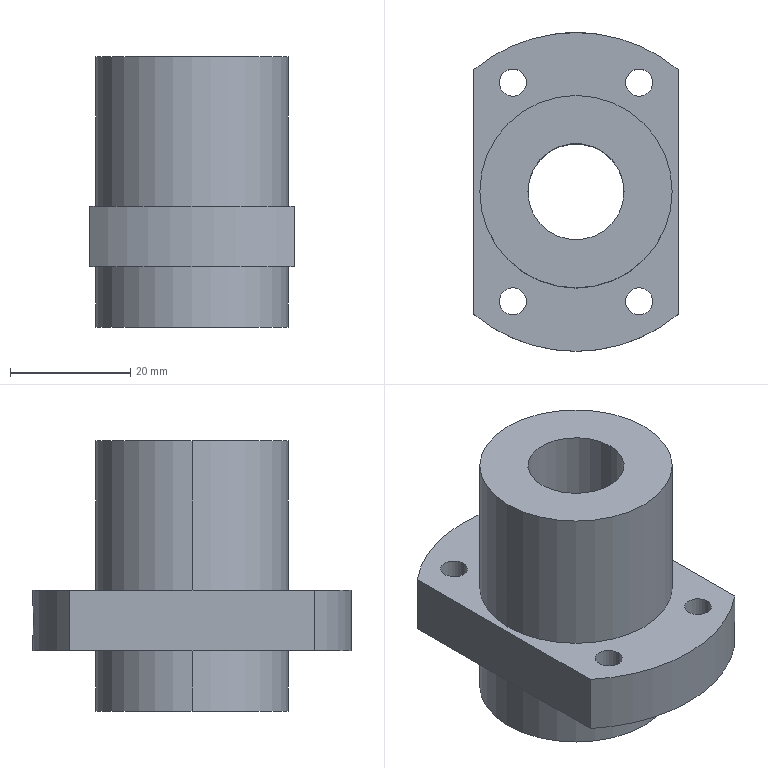Part | STEP file | HI_LCP02-16-16-L200-F15-P8_2 | 1 solid | 29 faces | box 34 x 53 x 45 mm | volume 34960 mm3 | cylinder 20 | plane 7 | cone 2 | commonest cylinder face diameters 4.5 x8 32 x4 3 x2 4.917 x2 16 x2 53 x2